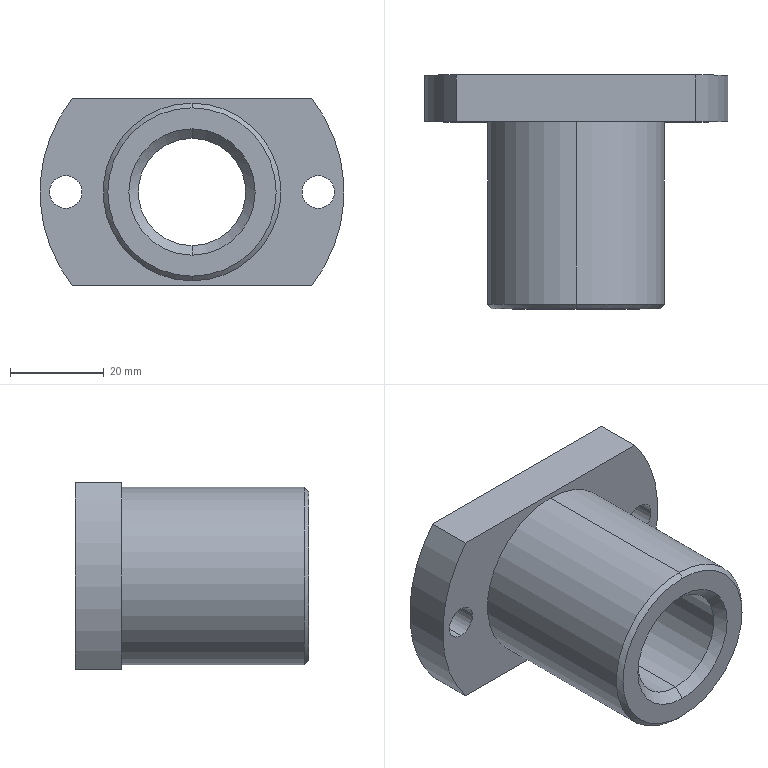Part | SolidWorks | features ICE 4, Chamfer 2, CirPattern 1, Extrusion 1 | 1 solid | 21 faces | box 65 x 50 x 40 mm | volume 47707 mm3 | cylinder 10 | cone 6 | plane 5 | commonest cylinder face diameters 7 x4 23 x2 38 x2 65 x2
STEP:
#1=CARTESIAN_POINT('',(0.,48.,-11.5));
#2=VERTEX_POINT('',#1);
#3=CARTESIAN_POINT('',(0.,48.,11.5));
#4=VERTEX_POINT('',#3);
#5=CARTESIAN_POINT('',(0.,48.,0.));
#6=DIRECTION('',(0.,1.,0.));
#7=DIRECTION('',(0.,0.,1.));
#8=AXIS2_PLACEMENT_3D('',#5,#6,#7);
#9=CIRCLE('',#8,11.5);
#10=EDGE_CURVE('',#2,#4,#9,.T.);
#11=ORIENTED_EDGE('',*,*,#10,.F.);
#12=CARTESIAN_POINT('',(0.,50.,-13.5));
#13=VERTEX_POINT('',#12);
#14=CARTESIAN_POINT('',(0.,50.,-13.5));
#15=DIRECTION('',(0.,0.7071,-0.7071));
#16=VECTOR('',#15,1000.);
#17=LINE('',#14,#16);
#18=EDGE_CURVE('',#2,#13,#17,.T.);
#19=ORIENTED_EDGE('',*,*,#18,.T.);
#20=CARTESIAN_POINT('',(0.,50.,13.5));
#21=VERTEX_POINT('',#20);
#22=CARTESIAN_POINT('',(0.,50.,0.));
#23=DIRECTION('',(0.,-1.,0.));
#24=DIRECTION('',(0.,0.,1.));
#25=AXIS2_PLACEMENT_3D('',#22,#23,#24);
#26=CIRCLE('',#25,13.5);
#27=EDGE_CURVE('',#21,#13,#26,.T.);
#28=ORIENTED_EDGE('',*,*,#27,.F.);
#29=CARTESIAN_POINT('',(0.,50.,13.5));
#30=DIRECTION('',(0.,0.7071,0.7071));
#31=VECTOR('',#30,1000.);
#32=LINE('',#29,#31);
#33=EDGE_CURVE('',#4,#21,#32,.T.);
#34=ORIENTED_EDGE('',*,*,#33,.F.);
#35=EDGE_LOOP('',(#11,#19,#28,#34));
#36=FACE_OUTER_BOUND('',#35,.T.);
#37=CARTESIAN_POINT('',(0.,50.,0.));
#38=DIRECTION('',(0.,1.,0.));
#39=DIRECTION('',(0.,0.,1.));
#40=AXIS2_PLACEMENT_3D('',#37,#38,#39);
#41=CONICAL_SURFACE('',#40,13.5,0.7854);
#42=ADVANCED_FACE('',(#36),#41,.F.);
#43=CARTESIAN_POINT('',(0.,2.,11.5));
#44=VERTEX_POINT('',#43);
#45=CARTESIAN_POINT('',(0.,2.,-11.5));
#46=VERTEX_POINT('',#45);
#47=CARTESIAN_POINT('',(0.,2.,0.));
#48=DIRECTION('',(0.,-1.,0.));
#49=DIRECTION('',(0.,0.,1.));
#50=AXIS2_PLACEMENT_3D('',#47,#48,#49);
#51=CIRCLE('',#50,11.5);
#52=EDGE_CURVE('',#44,#46,#51,.T.);
#53=ORIENTED_EDGE('',*,*,#52,.F.);
#54=CARTESIAN_POINT('',(0.,0.,13.5));
#55=VERTEX_POINT('',#54);
#56=CARTESIAN_POINT('',(0.,2.,11.5));
#57=DIRECTION('',(0.,-0.7071,0.7071));
#58=VECTOR('',#57,1000.);
#59=LINE('',#56,#58);
#60=EDGE_CURVE('',#44,#55,#59,.T.);
#61=ORIENTED_EDGE('',*,*,#60,.T.);
#62=CARTESIAN_POINT('',(0.,0.,-13.5));
#63=VERTEX_POINT('',#62);
#64=CARTESIAN_POINT('',(0.,0.,0.));
#65=DIRECTION('',(0.,1.,0.));
#66=DIRECTION('',(0.,0.,1.));
#67=AXIS2_PLACEMENT_3D('',#64,#65,#66);
#68=CIRCLE('',#67,13.5);
#69=EDGE_CURVE('',#63,#55,#68,.T.);
#70=ORIENTED_EDGE('',*,*,#69,.F.);
#71=CARTESIAN_POINT('',(0.,2.,-11.5));
#72=DIRECTION('',(0.,-0.7071,-0.7071));
#73=VECTOR('',#72,1000.);
#74=LINE('',#71,#73);
#75=EDGE_CURVE('',#46,#63,#74,.T.);
#76=ORIENTED_EDGE('',*,*,#75,.F.);
#77=EDGE_LOOP('',(#53,#61,#70,#76));
#78=FACE_OUTER_BOUND('',#77,.T.);
#79=CARTESIAN_POINT('',(0.,2.,0.));
#80=DIRECTION('',(0.,-1.,0.));
#81=DIRECTION('',(0.,0.,-1.));
#82=AXIS2_PLACEMENT_3D('',#79,#80,#81);
#83=CONICAL_SURFACE('',#82,11.5,0.7854);
#84=ADVANCED_FACE('',(#78),#83,.F.);
#85=CARTESIAN_POINT('',(0.,0.,-18.));
#86=VERTEX_POINT('',#85);
#87=CARTESIAN_POINT('',(0.,0.,18.));
#88=VERTEX_POINT('',#87);
#89=CARTESIAN_POINT('',(0.,0.,0.));
#90=DIRECTION('',(0.,-1.,0.));
#91=DIRECTION('',(0.,0.,1.));
#92=AXIS2_PLACEMENT_3D('',#89,#90,#91);
#93=CIRCLE('',#92,18.);
#94=EDGE_CURVE('',#86,#88,#93,.T.);
#95=ORIENTED_EDGE('',*,*,#94,.F.);
#96=CARTESIAN_POINT('',(0.,1.,-19.));
#97=VERTEX_POINT('',#96);
#98=CARTESIAN_POINT('',(0.,1.,-19.));
#99=DIRECTION('',(0.,0.7071,-0.7071));
#100=VECTOR('',#99,1000.);
#101=LINE('',#98,#100);
#102=EDGE_CURVE('',#86,#97,#101,.T.);
#103=ORIENTED_EDGE('',*,*,#102,.T.);
#104=CARTESIAN_POINT('',(0.,1.,19.));
#105=VERTEX_POINT('',#104);
#106=CARTESIAN_POINT('',(0.,1.,0.));
#107=DIRECTION('',(0.,1.,0.));
#108=DIRECTION('',(0.,0.,1.));
#109=AXIS2_PLACEMENT_3D('',#106,#107,#108);
#110=CIRCLE('',#109,19.);
#111=EDGE_CURVE('',#105,#97,#110,.T.);
#112=ORIENTED_EDGE('',*,*,#111,.F.);
#113=CARTESIAN_POINT('',(0.,1.,19.));
#114=DIRECTION('',(0.,0.7071,0.7071));
#115=VECTOR('',#114,1000.);
#116=LINE('',#113,#115);
#117=EDGE_CURVE('',#88,#105,#116,.T.);
#118=ORIENTED_EDGE('',*,*,#117,.F.);
#119=EDGE_LOOP('',(#95,#103,#112,#118));
#120=FACE_OUTER_BOUND('',#119,.T.);
#121=CARTESIAN_POINT('',(0.,1.,0.));
#122=DIRECTION('',(0.,1.,0.));
#123=DIRECTION('',(0.,0.,1.));
#124=AXIS2_PLACEMENT_3D('',#121,#122,#123);
#125=CONICAL_SURFACE('',#124,19.,0.7854);
#126=ADVANCED_FACE('',(#120),#125,.T.);
#127=CARTESIAN_POINT('',(27.,50.,3.5));
#128=VERTEX_POINT('',#127);
#129=CARTESIAN_POINT('',(27.,50.,-3.5));
#130=VERTEX_POINT('',#129);
#131=CARTESIAN_POINT('',(27.,50.,0.));
#132=DIRECTION('',(0.,-1.,0.));
#133=DIRECTION('',(0.,0.,1.));
#134=AXIS2_PLACEMENT_3D('',#131,#132,#133);
#135=CIRCLE('',#134,3.5);
#136=EDGE_CURVE('',#128,#130,#135,.T.);
#137=ORIENTED_EDGE('',*,*,#136,.F.);
#138=CARTESIAN_POINT('',(27.,40.,3.5));
#139=VERTEX_POINT('',#138);
#140=CARTESIAN_POINT('',(27.,50.,3.5));
#141=DIRECTION('',(0.,-1.,0.));
#142=VECTOR('',#141,1000.);
#143=LINE('',#140,#142);
#144=EDGE_CURVE('',#128,#139,#143,.T.);
#145=ORIENTED_EDGE('',*,*,#144,.T.);
#146=CARTESIAN_POINT('',(27.,40.,-3.5));
#147=VERTEX_POINT('',#146);
#148=CARTESIAN_POINT('',(27.,40.,0.));
#149=DIRECTION('',(0.,-1.,0.));
#150=DIRECTION('',(0.,0.,1.));
#151=AXIS2_PLACEMENT_3D('',#148,#149,#150);
#152=CIRCLE('',#151,3.5);
#153=EDGE_CURVE('',#139,#147,#152,.T.);
#154=ORIENTED_EDGE('',*,*,#153,.T.);
#155=CARTESIAN_POINT('',(27.,50.,-3.5));
#156=DIRECTION('',(0.,-1.,0.));
#157=VECTOR('',#156,1000.);
#158=LINE('',#155,#157);
#159=EDGE_CURVE('',#130,#147,#158,.T.);
#160=ORIENTED_EDGE('',*,*,#159,.F.);
#161=EDGE_LOOP('',(#137,#145,#154,#160));
#162=FACE_OUTER_BOUND('',#161,.T.);
#163=CARTESIAN_POINT('',(27.,50.,0.));
#164=DIRECTION('',(0.,-1.,0.));
#165=DIRECTION('',(0.,0.,-1.));
#166=AXIS2_PLACEMENT_3D('',#163,#164,#165);
#167=CYLINDRICAL_SURFACE('',#166,3.5);
#168=ADVANCED_FACE('',(#162),#167,.F.);
#169=CARTESIAN_POINT('',(-27.,50.,3.5));
#170=VERTEX_POINT('',#169);
#171=CARTESIAN_POINT('',(-27.,50.,-3.5));
#172=VERTEX_POINT('',#171);
#173=CARTESIAN_POINT('',(-27.,50.,0.));
#174=DIRECTION('',(0.,-1.,0.));
#175=DIRECTION('',(0.,0.,-1.));
#176=AXIS2_PLACEMENT_3D('',#173,#174,#175);
#177=CIRCLE('',#176,3.5);
#178=EDGE_CURVE('',#170,#172,#177,.T.);
#179=ORIENTED_EDGE('',*,*,#178,.F.);
#180=CARTESIAN_POINT('',(-27.,40.,3.5));
#181=VERTEX_POINT('',#180);
#182=CARTESIAN_POINT('',(-27.,50.,3.5));
#183=DIRECTION('',(0.,-1.,0.));
#184=VECTOR('',#183,1000.);
#185=LINE('',#182,#184);
#186=EDGE_CURVE('',#170,#181,#185,.T.);
#187=ORIENTED_EDGE('',*,*,#186,.T.);
#188=CARTESIAN_POINT('',(-27.,40.,-3.5));
#189=VERTEX_POINT('',#188);
#190=CARTESIAN_POINT('',(-27.,40.,0.));
#191=DIRECTION('',(0.,-1.,0.));
#192=DIRECTION('',(0.,0.,-1.));
#193=AXIS2_PLACEMENT_3D('',#190,#191,#192);
#194=CIRCLE('',#193,3.5);
#195=EDGE_CURVE('',#181,#189,#194,.T.);
#196=ORIENTED_EDGE('',*,*,#195,.T.);
#197=CARTESIAN_POINT('',(-27.,50.,-3.5));
#198=DIRECTION('',(0.,-1.,0.));
#199=VECTOR('',#198,1000.);
#200=LINE('',#197,#199);
#201=EDGE_CURVE('',#172,#189,#200,.T.);
#202=ORIENTED_EDGE('',*,*,#201,.F.);
#203=EDGE_LOOP('',(#179,#187,#196,#202));
#204=FACE_OUTER_BOUND('',#203,.T.);
#205=CARTESIAN_POINT('',(-27.,50.,0.));
#206=DIRECTION('',(0.,-1.,0.));
#207=DIRECTION('',(0.,0.,-1.));
#208=AXIS2_PLACEMENT_3D('',#205,#206,#207);
#209=CYLINDRICAL_SURFACE('',#208,3.5);
#210=ADVANCED_FACE('',(#204),#209,.F.);
#211=ORIENTED_EDGE('',*,*,#10,.T.);
#212=CARTESIAN_POINT('',(0.,50.001,11.5));
#213=DIRECTION('',(0.,-1.,0.));
#214=VECTOR('',#213,1000.);
#215=LINE('',#212,#214);
#216=EDGE_CURVE('',#4,#44,#215,.T.);
#217=ORIENTED_EDGE('',*,*,#216,.T.);
#218=ORIENTED_EDGE('',*,*,#52,.T.);
#219=CARTESIAN_POINT('',(0.,50.001,-11.5));
#220=DIRECTION('',(0.,-1.,0.));
#221=VECTOR('',#220,1000.);
#222=LINE('',#219,#221);
#223=EDGE_CURVE('',#2,#46,#222,.T.);
#224=ORIENTED_EDGE('',*,*,#223,.F.);
#225=EDGE_LOOP('',(#211,#217,#218,#224));
#226=FACE_OUTER_BOUND('',#225,.T.);
#227=CARTESIAN_POINT('',(0.,50.001,0.));
#228=DIRECTION('',(0.,-1.,0.));
#229=DIRECTION('',(0.,0.,-1.));
#230=AXIS2_PLACEMENT_3D('',#227,#228,#229);
#231=CYLINDRICAL_SURFACE('',#230,11.5);
#232=ADVANCED_FACE('',(#226),#231,.F.);
#233=CARTESIAN_POINT('',(0.,40.,19.));
#234=VERTEX_POINT('',#233);
#235=CARTESIAN_POINT('',(0.,40.,-19.));
#236=VERTEX_POINT('',#235);
#237=CARTESIAN_POINT('',(0.,40.,0.));
#238=DIRECTION('',(0.,1.,0.));
#239=DIRECTION('',(0.,0.,1.));
#240=AXIS2_PLACEMENT_3D('',#237,#238,#239);
#241=CIRCLE('',#240,19.);
#242=EDGE_CURVE('',#234,#236,#241,.T.);
#243=ORIENTED_EDGE('',*,*,#242,.F.);
#244=CARTESIAN_POINT('',(0.,50.,19.));
#245=DIRECTION('',(0.,-1.,0.));
#246=VECTOR('',#245,1000.);
#247=LINE('',#244,#246);
#248=EDGE_CURVE('',#234,#105,#247,.T.);
#249=ORIENTED_EDGE('',*,*,#248,.T.);
#250=ORIENTED_EDGE('',*,*,#111,.T.);
#251=CARTESIAN_POINT('',(0.,50.,-19.));
#252=DIRECTION('',(0.,-1.,0.));
#253=VECTOR('',#252,1000.);
#254=LINE('',#251,#253);
#255=EDGE_CURVE('',#236,#97,#254,.T.);
#256=ORIENTED_EDGE('',*,*,#255,.F.);
#257=EDGE_LOOP('',(#243,#249,#250,#256));
#258=FACE_OUTER_BOUND('',#257,.T.);
#259=CARTESIAN_POINT('',(0.,50.,0.));
#260=DIRECTION('',(0.,-1.,0.));
#261=DIRECTION('',(0.,0.,-1.));
#262=AXIS2_PLACEMENT_3D('',#259,#260,#261);
#263=CYLINDRICAL_SURFACE('',#262,19.);
#264=ADVANCED_FACE('',(#258),#263,.T.);
#265=CARTESIAN_POINT('',(25.617,40.,-20.));
#266=VERTEX_POINT('',#265);
#267=CARTESIAN_POINT('',(25.617,50.,-20.));
#268=VERTEX_POINT('',#267);
#269=CARTESIAN_POINT('',(25.617,-0.001,-20.));
#270=DIRECTION('',(0.,1.,0.));
#271=VECTOR('',#270,1000.);
#272=LINE('',#269,#271);
#273=EDGE_CURVE('',#266,#268,#272,.T.);
#274=ORIENTED_EDGE('',*,*,#273,.T.);
#275=CARTESIAN_POINT('',(25.617,50.,20.));
#276=VERTEX_POINT('',#275);
#277=CARTESIAN_POINT('',(0.,50.,0.));
#278=DIRECTION('',(0.,1.,0.));
#279=DIRECTION('',(0.,0.,1.));
#280=AXIS2_PLACEMENT_3D('',#277,#278,#279);
#281=CIRCLE('',#280,32.5);
#282=EDGE_CURVE('',#276,#268,#281,.T.);
#283=ORIENTED_EDGE('',*,*,#282,.F.);
#284=CARTESIAN_POINT('',(25.617,40.,20.));
#285=VERTEX_POINT('',#284);
#286=CARTESIAN_POINT('',(25.617,-0.001,20.));
#287=DIRECTION('',(0.,1.,0.));
#288=VECTOR('',#287,1000.);
#289=LINE('',#286,#288);
#290=EDGE_CURVE('',#285,#276,#289,.T.);
#291=ORIENTED_EDGE('',*,*,#290,.F.);
#292=CARTESIAN_POINT('',(0.,40.,0.));
#293=DIRECTION('',(0.,1.,0.));
#294=DIRECTION('',(0.,0.,1.));
#295=AXIS2_PLACEMENT_3D('',#292,#293,#294);
#296=CIRCLE('',#295,32.5);
#297=EDGE_CURVE('',#285,#266,#296,.T.);
#298=ORIENTED_EDGE('',*,*,#297,.T.);
#299=EDGE_LOOP('',(#274,#283,#291,#298));
#300=FACE_OUTER_BOUND('',#299,.T.);
#301=CARTESIAN_POINT('',(0.,40.,0.));
#302=DIRECTION('',(0.,1.,0.));
#303=DIRECTION('',(0.,0.,1.));
#304=AXIS2_PLACEMENT_3D('',#301,#302,#303);
#305=CYLINDRICAL_SURFACE('',#304,32.5);
#306=ADVANCED_FACE('',(#300),#305,.T.);
#307=ORIENTED_EDGE('',*,*,#248,.F.);
#308=CARTESIAN_POINT('',(0.,40.,0.));
#309=DIRECTION('',(0.,1.,0.));
#310=DIRECTION('',(0.,0.,1.));
#311=AXIS2_PLACEMENT_3D('',#308,#309,#310);
#312=CIRCLE('',#311,19.);
#313=EDGE_CURVE('',#236,#234,#312,.T.);
#314=ORIENTED_EDGE('',*,*,#313,.F.);
#315=ORIENTED_EDGE('',*,*,#255,.T.);
#316=CARTESIAN_POINT('',(0.,1.,0.));
#317=DIRECTION('',(0.,1.,0.));
#318=DIRECTION('',(0.,0.,1.));
#319=AXIS2_PLACEMENT_3D('',#316,#317,#318);
#320=CIRCLE('',#319,19.);
#321=EDGE_CURVE('',#97,#105,#320,.T.);
#322=ORIENTED_EDGE('',*,*,#321,.T.);
#323=EDGE_LOOP('',(#307,#314,#315,#322));
#324=FACE_OUTER_BOUND('',#323,.T.);
#325=CARTESIAN_POINT('',(0.,50.,0.));
#326=DIRECTION('',(0.,-1.,0.));
#327=DIRECTION('',(0.,0.,-1.));
#328=AXIS2_PLACEMENT_3D('',#325,#326,#327);
#329=CYLINDRICAL_SURFACE('',#328,19.);
#330=ADVANCED_FACE('',(#324),#329,.T.);
#331=ORIENTED_EDGE('',*,*,#69,.T.);
#332=CARTESIAN_POINT('',(0.,0.,0.));
#333=DIRECTION('',(0.,1.,0.));
#334=DIRECTION('',(0.,0.,1.));
#335=AXIS2_PLACEMENT_3D('',#332,#333,#334);
#336=CIRCLE('',#335,13.5);
#337=EDGE_CURVE('',#55,#63,#336,.T.);
#338=ORIENTED_EDGE('',*,*,#337,.T.);
#339=EDGE_LOOP('',(#331,#338));
#340=FACE_BOUND('',#339,.T.);
#341=CARTESIAN_POINT('',(0.,0.,0.));
#342=DIRECTION('',(0.,-1.,0.));
#343=DIRECTION('',(0.,0.,1.));
#344=AXIS2_PLACEMENT_3D('',#341,#342,#343);
#345=CIRCLE('',#344,18.);
#346=EDGE_CURVE('',#88,#86,#345,.T.);
#347=ORIENTED_EDGE('',*,*,#346,.T.);
#348=ORIENTED_EDGE('',*,*,#94,.T.);
#349=EDGE_LOOP('',(#347,#348));
#350=FACE_OUTER_BOUND('',#349,.T.);
#351=CARTESIAN_POINT('',(0.,0.,0.));
#352=DIRECTION('',(0.,1.,0.));
#353=DIRECTION('',(0.,0.,1.));
#354=AXIS2_PLACEMENT_3D('',#351,#352,#353);
#355=PLANE('',#354);
#356=ADVANCED_FACE('',(#340,#350),#355,.F.);
#357=CARTESIAN_POINT('',(-25.617,40.,-20.));
#358=VERTEX_POINT('',#357);
#359=CARTESIAN_POINT('',(-25.617,50.,-20.));
#360=VERTEX_POINT('',#359);
#361=CARTESIAN_POINT('',(-25.617,-0.001,-20.));
#362=DIRECTION('',(0.,1.,0.));
#363=VECTOR('',#362,1000.);
#364=LINE('',#361,#363);
#365=EDGE_CURVE('',#358,#360,#364,.T.);
#366=ORIENTED_EDGE('',*,*,#365,.F.);
#367=CARTESIAN_POINT('',(-25.617,40.,20.));
#368=VERTEX_POINT('',#367);
#369=CARTESIAN_POINT('',(0.,40.,0.));
#370=DIRECTION('',(0.,1.,0.));
#371=DIRECTION('',(0.,0.,1.));
#372=AXIS2_PLACEMENT_3D('',#369,#370,#371);
#373=CIRCLE('',#372,32.5);
#374=EDGE_CURVE('',#358,#368,#373,.T.);
#375=ORIENTED_EDGE('',*,*,#374,.T.);
#376=CARTESIAN_POINT('',(-25.617,50.,20.));
#377=VERTEX_POINT('',#376);
#378=CARTESIAN_POINT('',(-25.617,-0.001,20.));
#379=DIRECTION('',(0.,1.,0.));
#380=VECTOR('',#379,1000.);
#381=LINE('',#378,#380);
#382=EDGE_CURVE('',#368,#377,#381,.T.);
#383=ORIENTED_EDGE('',*,*,#382,.T.);
#384=CARTESIAN_POINT('',(0.,50.,0.));
#385=DIRECTION('',(0.,1.,0.));
#386=DIRECTION('',(0.,0.,1.));
#387=AXIS2_PLACEMENT_3D('',#384,#385,#386);
#388=CIRCLE('',#387,32.5);
#389=EDGE_CURVE('',#360,#377,#388,.T.);
#390=ORIENTED_EDGE('',*,*,#389,.F.);
#391=EDGE_LOOP('',(#366,#375,#383,#390));
#392=FACE_OUTER_BOUND('',#391,.T.);
#393=CARTESIAN_POINT('',(0.,40.,0.));
#394=DIRECTION('',(0.,1.,0.));
#395=DIRECTION('',(0.,0.,1.));
#396=AXIS2_PLACEMENT_3D('',#393,#394,#395);
#397=CYLINDRICAL_SURFACE('',#396,32.5);
#398=ADVANCED_FACE('',(#392),#397,.T.);
#399=CARTESIAN_POINT('',(27.,40.,0.));
#400=DIRECTION('',(0.,-1.,0.));
#401=DIRECTION('',(0.,0.,1.));
#402=AXIS2_PLACEMENT_3D('',#399,#400,#401);
#403=CIRCLE('',#402,3.5);
#404=EDGE_CURVE('',#147,#139,#403,.T.);
#405=ORIENTED_EDGE('',*,*,#404,.F.);
#406=ORIENTED_EDGE('',*,*,#153,.F.);
#407=EDGE_LOOP('',(#405,#406));
#408=FACE_BOUND('',#407,.T.);
#409=CARTESIAN_POINT('',(-27.,40.,0.));
#410=DIRECTION('',(0.,-1.,0.));
#411=DIRECTION('',(0.,0.,-1.));
#412=AXIS2_PLACEMENT_3D('',#409,#410,#411);
#413=CIRCLE('',#412,3.5);
#414=EDGE_CURVE('',#189,#181,#413,.T.);
#415=ORIENTED_EDGE('',*,*,#414,.F.);
#416=ORIENTED_EDGE('',*,*,#195,.F.);
#417=EDGE_LOOP('',(#415,#416));
#418=FACE_BOUND('',#417,.T.);
#419=ORIENTED_EDGE('',*,*,#313,.T.);
#420=ORIENTED_EDGE('',*,*,#242,.T.);
#421=EDGE_LOOP('',(#419,#420));
#422=FACE_BOUND('',#421,.T.);
#423=ORIENTED_EDGE('',*,*,#374,.F.);
#424=CARTESIAN_POINT('',(-25.617,40.,-20.));
#425=DIRECTION('',(-1.,0.,0.));
#426=VECTOR('',#425,1000.);
#427=LINE('',#424,#426);
#428=EDGE_CURVE('',#266,#358,#427,.T.);
#429=ORIENTED_EDGE('',*,*,#428,.F.);
#430=ORIENTED_EDGE('',*,*,#297,.F.);
#431=CARTESIAN_POINT('',(-25.617,40.,20.));
#432=DIRECTION('',(1.,0.,0.));
#433=VECTOR('',#432,1000.);
#434=LINE('',#431,#433);
#435=EDGE_CURVE('',#368,#285,#434,.T.);
#436=ORIENTED_EDGE('',*,*,#435,.F.);
#437=EDGE_LOOP('',(#423,#429,#430,#436));
#438=FACE_OUTER_BOUND('',#437,.T.);
#439=CARTESIAN_POINT('',(0.,40.,0.));
#440=DIRECTION('',(0.,1.,0.));
#441=DIRECTION('',(0.,0.,1.));
#442=AXIS2_PLACEMENT_3D('',#439,#440,#441);
#443=PLANE('',#442);
#444=ADVANCED_FACE('',(#408,#418,#422,#438),#443,.F.);
#445=CARTESIAN_POINT('',(-25.617,50.,-20.));
#446=DIRECTION('',(1.,0.,0.));
#447=VECTOR('',#446,1000.);
#448=LINE('',#445,#447);
#449=EDGE_CURVE('',#360,#268,#448,.T.);
#450=ORIENTED_EDGE('',*,*,#449,.F.);
#451=ORIENTED_EDGE('',*,*,#389,.T.);
#452=CARTESIAN_POINT('',(-25.617,50.,20.));
#453=DIRECTION('',(-1.,0.,0.));
#454=VECTOR('',#453,1000.);
#455=LINE('',#452,#454);
#456=EDGE_CURVE('',#276,#377,#455,.T.);
#457=ORIENTED_EDGE('',*,*,#456,.F.);
#458=ORIENTED_EDGE('',*,*,#282,.T.);
#459=EDGE_LOOP('',(#450,#451,#457,#458));
#460=FACE_OUTER_BOUND('',#459,.T.);
#461=ORIENTED_EDGE('',*,*,#27,.T.);
#462=CARTESIAN_POINT('',(0.,50.,0.));
#463=DIRECTION('',(0.,-1.,0.));
#464=DIRECTION('',(0.,0.,1.));
#465=AXIS2_PLACEMENT_3D('',#462,#463,#464);
#466=CIRCLE('',#465,13.5);
#467=EDGE_CURVE('',#13,#21,#466,.T.);
#468=ORIENTED_EDGE('',*,*,#467,.T.);
#469=EDGE_LOOP('',(#461,#468));
#470=FACE_BOUND('',#469,.T.);
#471=CARTESIAN_POINT('',(27.,50.,0.));
#472=DIRECTION('',(0.,-1.,0.));
#473=DIRECTION('',(0.,0.,1.));
#474=AXIS2_PLACEMENT_3D('',#471,#472,#473);
#475=CIRCLE('',#474,3.5);
#476=EDGE_CURVE('',#130,#128,#475,.T.);
#477=ORIENTED_EDGE('',*,*,#476,.T.);
#478=ORIENTED_EDGE('',*,*,#136,.T.);
#479=EDGE_LOOP('',(#477,#478));
#480=FACE_BOUND('',#479,.T.);
#481=CARTESIAN_POINT('',(-27.,50.,0.));
#482=DIRECTION('',(0.,-1.,0.));
#483=DIRECTION('',(0.,0.,-1.));
#484=AXIS2_PLACEMENT_3D('',#481,#482,#483);
#485=CIRCLE('',#484,3.5);
#486=EDGE_CURVE('',#172,#170,#485,.T.);
#487=ORIENTED_EDGE('',*,*,#486,.T.);
#488=ORIENTED_EDGE('',*,*,#178,.T.);
#489=EDGE_LOOP('',(#487,#488));
#490=FACE_BOUND('',#489,.T.);
#491=CARTESIAN_POINT('',(0.,50.,0.));
#492=DIRECTION('',(0.,1.,0.));
#493=DIRECTION('',(0.,0.,1.));
#494=AXIS2_PLACEMENT_3D('',#491,#492,#493);
#495=PLANE('',#494);
#496=ADVANCED_FACE('',(#460,#470,#480,#490),#495,.T.);
#497=ORIENTED_EDGE('',*,*,#216,.F.);
#498=CARTESIAN_POINT('',(0.,48.,0.));
#499=DIRECTION('',(0.,1.,0.));
#500=DIRECTION('',(0.,0.,1.));
#501=AXIS2_PLACEMENT_3D('',#498,#499,#500);
#502=CIRCLE('',#501,11.5);
#503=EDGE_CURVE('',#4,#2,#502,.T.);
#504=ORIENTED_EDGE('',*,*,#503,.T.);
#505=ORIENTED_EDGE('',*,*,#223,.T.);
#506=CARTESIAN_POINT('',(0.,2.,0.));
#507=DIRECTION('',(0.,-1.,0.));
#508=DIRECTION('',(0.,0.,1.));
#509=AXIS2_PLACEMENT_3D('',#506,#507,#508);
#510=CIRCLE('',#509,11.5);
#511=EDGE_CURVE('',#46,#44,#510,.T.);
#512=ORIENTED_EDGE('',*,*,#511,.T.);
#513=EDGE_LOOP('',(#497,#504,#505,#512));
#514=FACE_OUTER_BOUND('',#513,.T.);
#515=CARTESIAN_POINT('',(0.,50.001,0.));
#516=DIRECTION('',(0.,-1.,0.));
#517=DIRECTION('',(0.,0.,-1.));
#518=AXIS2_PLACEMENT_3D('',#515,#516,#517);
#519=CYLINDRICAL_SURFACE('',#518,11.5);
#520=ADVANCED_FACE('',(#514),#519,.F.);
#521=ORIENTED_EDGE('',*,*,#186,.F.);
#522=ORIENTED_EDGE('',*,*,#486,.F.);
#523=ORIENTED_EDGE('',*,*,#201,.T.);
#524=ORIENTED_EDGE('',*,*,#414,.T.);
#525=EDGE_LOOP('',(#521,#522,#523,#524));
#526=FACE_OUTER_BOUND('',#525,.T.);
#527=CARTESIAN_POINT('',(-27.,50.,0.));
#528=DIRECTION('',(0.,-1.,0.));
#529=DIRECTION('',(0.,0.,-1.));
#530=AXIS2_PLACEMENT_3D('',#527,#528,#529);
#531=CYLINDRICAL_SURFACE('',#530,3.5);
#532=ADVANCED_FACE('',(#526),#531,.F.);
#533=ORIENTED_EDGE('',*,*,#144,.F.);
#534=ORIENTED_EDGE('',*,*,#476,.F.);
#535=ORIENTED_EDGE('',*,*,#159,.T.);
#536=ORIENTED_EDGE('',*,*,#404,.T.);
#537=EDGE_LOOP('',(#533,#534,#535,#536));
#538=FACE_OUTER_BOUND('',#537,.T.);
#539=CARTESIAN_POINT('',(27.,50.,0.));
#540=DIRECTION('',(0.,-1.,0.));
#541=DIRECTION('',(0.,0.,-1.));
#542=AXIS2_PLACEMENT_3D('',#539,#540,#541);
#543=CYLINDRICAL_SURFACE('',#542,3.5);
#544=ADVANCED_FACE('',(#538),#543,.F.);
#545=ORIENTED_EDGE('',*,*,#102,.F.);
#546=ORIENTED_EDGE('',*,*,#346,.F.);
#547=ORIENTED_EDGE('',*,*,#117,.T.);
#548=ORIENTED_EDGE('',*,*,#321,.F.);
#549=EDGE_LOOP('',(#545,#546,#547,#548));
#550=FACE_OUTER_BOUND('',#549,.T.);
#551=CARTESIAN_POINT('',(0.,1.,0.));
#552=DIRECTION('',(0.,1.,0.));
#553=DIRECTION('',(0.,0.,1.));
#554=AXIS2_PLACEMENT_3D('',#551,#552,#553);
#555=CONICAL_SURFACE('',#554,19.,0.7854);
#556=ADVANCED_FACE('',(#550),#555,.T.);
#557=ORIENTED_EDGE('',*,*,#60,.F.);
#558=ORIENTED_EDGE('',*,*,#511,.F.);
#559=ORIENTED_EDGE('',*,*,#75,.T.);
#560=ORIENTED_EDGE('',*,*,#337,.F.);
#561=EDGE_LOOP('',(#557,#558,#559,#560));
#562=FACE_OUTER_BOUND('',#561,.T.);
#563=CARTESIAN_POINT('',(0.,2.,0.));
#564=DIRECTION('',(0.,-1.,0.));
#565=DIRECTION('',(0.,0.,-1.));
#566=AXIS2_PLACEMENT_3D('',#563,#564,#565);
#567=CONICAL_SURFACE('',#566,11.5,0.7854);
#568=ADVANCED_FACE('',(#562),#567,.F.);
#569=ORIENTED_EDGE('',*,*,#18,.F.);
#570=ORIENTED_EDGE('',*,*,#503,.F.);
#571=ORIENTED_EDGE('',*,*,#33,.T.);
#572=ORIENTED_EDGE('',*,*,#467,.F.);
#573=EDGE_LOOP('',(#569,#570,#571,#572));
#574=FACE_OUTER_BOUND('',#573,.T.);
#575=CARTESIAN_POINT('',(0.,50.,0.));
#576=DIRECTION('',(0.,1.,0.));
#577=DIRECTION('',(0.,0.,1.));
#578=AXIS2_PLACEMENT_3D('',#575,#576,#577);
#579=CONICAL_SURFACE('',#578,13.5,0.7854);
#580=ADVANCED_FACE('',(#574),#579,.F.);
#581=ORIENTED_EDGE('',*,*,#435,.T.);
#582=ORIENTED_EDGE('',*,*,#290,.T.);
#583=ORIENTED_EDGE('',*,*,#456,.T.);
#584=ORIENTED_EDGE('',*,*,#382,.F.);
#585=EDGE_LOOP('',(#581,#582,#583,#584));
#586=FACE_OUTER_BOUND('',#585,.T.);
#587=CARTESIAN_POINT('',(-25.617,-0.001,20.));
#588=DIRECTION('',(0.,0.,-1.));
#589=DIRECTION('',(-1.,0.,0.));
#590=AXIS2_PLACEMENT_3D('',#587,#588,#589);
#591=PLANE('',#590);
#592=ADVANCED_FACE('',(#586),#591,.F.);
#593=ORIENTED_EDGE('',*,*,#428,.T.);
#594=ORIENTED_EDGE('',*,*,#365,.T.);
#595=ORIENTED_EDGE('',*,*,#449,.T.);
#596=ORIENTED_EDGE('',*,*,#273,.F.);
#597=EDGE_LOOP('',(#593,#594,#595,#596));
#598=FACE_OUTER_BOUND('',#597,.T.);
#599=CARTESIAN_POINT('',(-25.617,-0.001,-20.));
#600=DIRECTION('',(0.,0.,1.));
#601=DIRECTION('',(1.,0.,0.));
#602=AXIS2_PLACEMENT_3D('',#599,#600,#601);
#603=PLANE('',#602);
#604=ADVANCED_FACE('',(#598),#603,.F.);
#605=CLOSED_SHELL('',(#42,#84,#126,#168,#210,#232,#264,#306,#330,#356,#398,#444,#496,#520,#532,#544,#556,#568,#580,#592,#604));
#606=MANIFOLD_SOLID_BREP('',#605);
#607=CARTESIAN_POINT('',(0.,0.,0.));
#608=DIRECTION('',(0.,0.,1.));
#609=DIRECTION('',(1.,0.,0.));
#610=AXIS2_PLACEMENT_3D('',#607,#608,#609);
#611=(LENGTH_UNIT()NAMED_UNIT(*)SI_UNIT(.MILLI.,.METRE.));
#612=UNCERTAINTY_MEASURE_WITH_UNIT(LENGTH_MEASURE(0.00001),#611,'','');
#613=(NAMED_UNIT(*)PLANE_ANGLE_UNIT()SI_UNIT($,.RADIAN.));
#614=(NAMED_UNIT(*)SI_UNIT($,.STERADIAN.)SOLID_ANGLE_UNIT());
#615=(GEOMETRIC_REPRESENTATION_CONTEXT(3)GLOBAL_UNCERTAINTY_ASSIGNED_CONTEXT((#612))GLOBAL_UNIT_ASSIGNED_CONTEXT((#611,#613,#614))REPRESENTATION_CONTEXT('',''));
#616=ADVANCED_BREP_SHAPE_REPRESENTATION('',(#606,#610),#615);